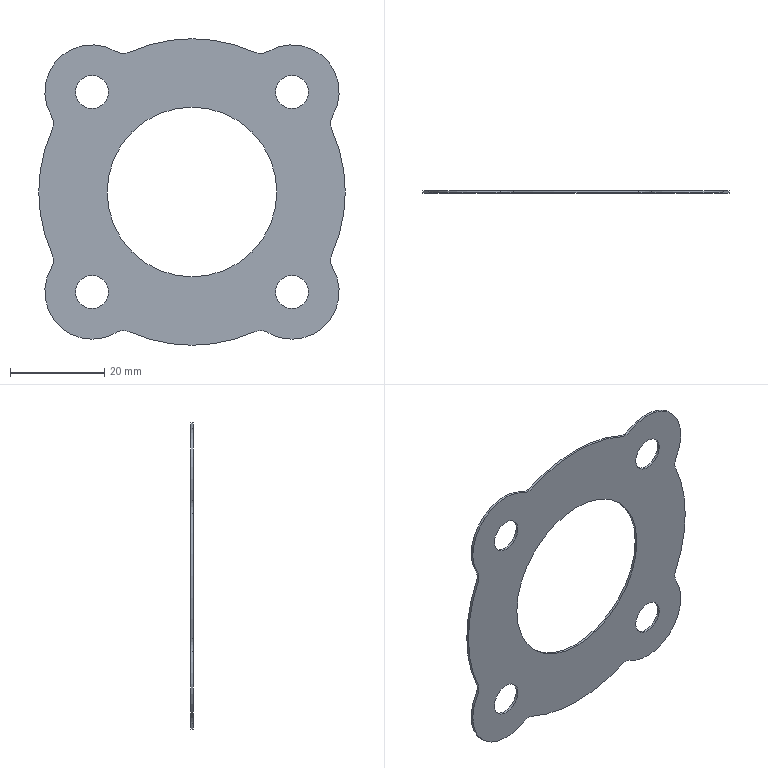Part | SolidWorks | features Extrusion 1, Fillet 1, ICE 1 | 1 solid | 33 faces | box 65 x 0.5 x 65 mm | volume 1310 mm3 | cylinder 31 | plane 2 | commonest cylinder face diameters 6 x10 7 x8 20 x6 65 x5 36 x2
STEP:
#1=CARTESIAN_POINT('',(14.555,0.,-29.379));
#2=VERTEX_POINT('',#1);
#3=CARTESIAN_POINT('',(16.092,0.,-29.802));
#4=VERTEX_POINT('',#3);
#5=CARTESIAN_POINT('',(14.555,0.,-32.379));
#6=DIRECTION('',(0.,1.,0.));
#7=DIRECTION('',(0.,0.,1.));
#8=AXIS2_PLACEMENT_3D('',#5,#6,#7);
#9=CIRCLE('',#8,3.);
#10=EDGE_CURVE('',#2,#4,#9,.T.);
#11=ORIENTED_EDGE('',*,*,#10,.F.);
#12=CARTESIAN_POINT('',(14.555,0.5,-29.379));
#13=VERTEX_POINT('',#12);
#14=CARTESIAN_POINT('',(14.555,0.5,-29.379));
#15=DIRECTION('',(0.,1.,0.));
#16=VECTOR('',#15,1000.);
#17=LINE('',#14,#16);
#18=EDGE_CURVE('',#2,#13,#17,.T.);
#19=ORIENTED_EDGE('',*,*,#18,.T.);
#20=CARTESIAN_POINT('',(16.092,0.5,-29.802));
#21=VERTEX_POINT('',#20);
#22=CARTESIAN_POINT('',(14.555,0.5,-32.379));
#23=DIRECTION('',(0.,-1.,0.));
#24=DIRECTION('',(0.,0.,1.));
#25=AXIS2_PLACEMENT_3D('',#22,#23,#24);
#26=CIRCLE('',#25,3.);
#27=EDGE_CURVE('',#21,#13,#26,.T.);
#28=ORIENTED_EDGE('',*,*,#27,.F.);
#29=CARTESIAN_POINT('',(16.092,0.5,-29.802));
#30=DIRECTION('',(0.,1.,0.));
#31=VECTOR('',#30,1000.);
#32=LINE('',#29,#31);
#33=EDGE_CURVE('',#4,#21,#32,.T.);
#34=ORIENTED_EDGE('',*,*,#33,.F.);
#35=EDGE_LOOP('',(#11,#19,#28,#34));
#36=FACE_OUTER_BOUND('',#35,.T.);
#37=CARTESIAN_POINT('',(14.555,0.5,-32.379));
#38=DIRECTION('',(0.,1.,0.));
#39=DIRECTION('',(0.,0.,1.));
#40=AXIS2_PLACEMENT_3D('',#37,#38,#39);
#41=CYLINDRICAL_SURFACE('',#40,3.);
#42=ADVANCED_FACE('',(#36),#41,.F.);
#43=CARTESIAN_POINT('',(-14.555,0.,-29.379));
#44=VERTEX_POINT('',#43);
#45=CARTESIAN_POINT('',(-13.325,0.,-29.643));
#46=VERTEX_POINT('',#45);
#47=CARTESIAN_POINT('',(-14.555,0.,-32.379));
#48=DIRECTION('',(0.,1.,0.));
#49=DIRECTION('',(0.,0.,1.));
#50=AXIS2_PLACEMENT_3D('',#47,#48,#49);
#51=CIRCLE('',#50,3.);
#52=EDGE_CURVE('',#44,#46,#51,.T.);
#53=ORIENTED_EDGE('',*,*,#52,.F.);
#54=CARTESIAN_POINT('',(-14.555,0.5,-29.379));
#55=VERTEX_POINT('',#54);
#56=CARTESIAN_POINT('',(-14.555,0.5,-29.379));
#57=DIRECTION('',(0.,1.,0.));
#58=VECTOR('',#57,1000.);
#59=LINE('',#56,#58);
#60=EDGE_CURVE('',#44,#55,#59,.T.);
#61=ORIENTED_EDGE('',*,*,#60,.T.);
#62=CARTESIAN_POINT('',(-13.325,0.5,-29.643));
#63=VERTEX_POINT('',#62);
#64=CARTESIAN_POINT('',(-14.555,0.5,-32.379));
#65=DIRECTION('',(0.,-1.,0.));
#66=DIRECTION('',(0.,0.,1.));
#67=AXIS2_PLACEMENT_3D('',#64,#65,#66);
#68=CIRCLE('',#67,3.);
#69=EDGE_CURVE('',#63,#55,#68,.T.);
#70=ORIENTED_EDGE('',*,*,#69,.F.);
#71=CARTESIAN_POINT('',(-13.325,0.5,-29.643));
#72=DIRECTION('',(0.,1.,0.));
#73=VECTOR('',#72,1000.);
#74=LINE('',#71,#73);
#75=EDGE_CURVE('',#46,#63,#74,.T.);
#76=ORIENTED_EDGE('',*,*,#75,.F.);
#77=EDGE_LOOP('',(#53,#61,#70,#76));
#78=FACE_OUTER_BOUND('',#77,.T.);
#79=CARTESIAN_POINT('',(-14.555,0.5,-32.379));
#80=DIRECTION('',(0.,1.,0.));
#81=DIRECTION('',(0.,0.,1.));
#82=AXIS2_PLACEMENT_3D('',#79,#80,#81);
#83=CYLINDRICAL_SURFACE('',#82,3.);
#84=ADVANCED_FACE('',(#78),#83,.F.);
#85=CARTESIAN_POINT('',(-21.213,0.,-24.713));
#86=VERTEX_POINT('',#85);
#87=CARTESIAN_POINT('',(-21.213,0.,-17.713));
#88=VERTEX_POINT('',#87);
#89=CARTESIAN_POINT('',(-21.213,0.,-21.213));
#90=DIRECTION('',(0.,1.,0.));
#91=DIRECTION('',(0.,0.,1.));
#92=AXIS2_PLACEMENT_3D('',#89,#90,#91);
#93=CIRCLE('',#92,3.5);
#94=EDGE_CURVE('',#86,#88,#93,.T.);
#95=ORIENTED_EDGE('',*,*,#94,.F.);
#96=CARTESIAN_POINT('',(-21.213,0.5,-24.713));
#97=VERTEX_POINT('',#96);
#98=CARTESIAN_POINT('',(-21.213,-49.5,-24.713));
#99=DIRECTION('',(0.,1.,0.));
#100=VECTOR('',#99,1000.);
#101=LINE('',#98,#100);
#102=EDGE_CURVE('',#86,#97,#101,.T.);
#103=ORIENTED_EDGE('',*,*,#102,.T.);
#104=CARTESIAN_POINT('',(-21.213,0.5,-17.713));
#105=VERTEX_POINT('',#104);
#106=CARTESIAN_POINT('',(-21.213,0.5,-21.213));
#107=DIRECTION('',(0.,1.,0.));
#108=DIRECTION('',(0.,0.,1.));
#109=AXIS2_PLACEMENT_3D('',#106,#107,#108);
#110=CIRCLE('',#109,3.5);
#111=EDGE_CURVE('',#97,#105,#110,.T.);
#112=ORIENTED_EDGE('',*,*,#111,.T.);
#113=CARTESIAN_POINT('',(-21.213,-49.5,-17.713));
#114=DIRECTION('',(0.,1.,0.));
#115=VECTOR('',#114,1000.);
#116=LINE('',#113,#115);
#117=EDGE_CURVE('',#88,#105,#116,.T.);
#118=ORIENTED_EDGE('',*,*,#117,.F.);
#119=EDGE_LOOP('',(#95,#103,#112,#118));
#120=FACE_OUTER_BOUND('',#119,.T.);
#121=CARTESIAN_POINT('',(-21.213,-49.5,-21.213));
#122=DIRECTION('',(0.,1.,0.));
#123=DIRECTION('',(0.,0.,1.));
#124=AXIS2_PLACEMENT_3D('',#121,#122,#123);
#125=CYLINDRICAL_SURFACE('',#124,3.5);
#126=ADVANCED_FACE('',(#120),#125,.F.);
#127=CARTESIAN_POINT('',(-21.213,0.,17.713));
#128=VERTEX_POINT('',#127);
#129=CARTESIAN_POINT('',(-21.213,0.,24.713));
#130=VERTEX_POINT('',#129);
#131=CARTESIAN_POINT('',(-21.213,0.,21.213));
#132=DIRECTION('',(0.,1.,0.));
#133=DIRECTION('',(0.,0.,1.));
#134=AXIS2_PLACEMENT_3D('',#131,#132,#133);
#135=CIRCLE('',#134,3.5);
#136=EDGE_CURVE('',#128,#130,#135,.T.);
#137=ORIENTED_EDGE('',*,*,#136,.F.);
#138=CARTESIAN_POINT('',(-21.213,0.5,17.713));
#139=VERTEX_POINT('',#138);
#140=CARTESIAN_POINT('',(-21.213,-49.5,17.713));
#141=DIRECTION('',(0.,1.,0.));
#142=VECTOR('',#141,1000.);
#143=LINE('',#140,#142);
#144=EDGE_CURVE('',#128,#139,#143,.T.);
#145=ORIENTED_EDGE('',*,*,#144,.T.);
#146=CARTESIAN_POINT('',(-21.213,0.5,24.713));
#147=VERTEX_POINT('',#146);
#148=CARTESIAN_POINT('',(-21.213,0.5,21.213));
#149=DIRECTION('',(0.,1.,0.));
#150=DIRECTION('',(0.,0.,1.));
#151=AXIS2_PLACEMENT_3D('',#148,#149,#150);
#152=CIRCLE('',#151,3.5);
#153=EDGE_CURVE('',#139,#147,#152,.T.);
#154=ORIENTED_EDGE('',*,*,#153,.T.);
#155=CARTESIAN_POINT('',(-21.213,-49.5,24.713));
#156=DIRECTION('',(0.,1.,0.));
#157=VECTOR('',#156,1000.);
#158=LINE('',#155,#157);
#159=EDGE_CURVE('',#130,#147,#158,.T.);
#160=ORIENTED_EDGE('',*,*,#159,.F.);
#161=EDGE_LOOP('',(#137,#145,#154,#160));
#162=FACE_OUTER_BOUND('',#161,.T.);
#163=CARTESIAN_POINT('',(-21.213,-49.5,21.213));
#164=DIRECTION('',(0.,1.,0.));
#165=DIRECTION('',(0.,0.,1.));
#166=AXIS2_PLACEMENT_3D('',#163,#164,#165);
#167=CYLINDRICAL_SURFACE('',#166,3.5);
#168=ADVANCED_FACE('',(#162),#167,.F.);
#169=CARTESIAN_POINT('',(21.213,0.,17.713));
#170=VERTEX_POINT('',#169);
#171=CARTESIAN_POINT('',(21.213,0.,24.713));
#172=VERTEX_POINT('',#171);
#173=CARTESIAN_POINT('',(21.213,0.,21.213));
#174=DIRECTION('',(0.,1.,0.));
#175=DIRECTION('',(0.,0.,1.));
#176=AXIS2_PLACEMENT_3D('',#173,#174,#175);
#177=CIRCLE('',#176,3.5);
#178=EDGE_CURVE('',#170,#172,#177,.T.);
#179=ORIENTED_EDGE('',*,*,#178,.F.);
#180=CARTESIAN_POINT('',(21.213,0.5,17.713));
#181=VERTEX_POINT('',#180);
#182=CARTESIAN_POINT('',(21.213,-49.5,17.713));
#183=DIRECTION('',(0.,1.,0.));
#184=VECTOR('',#183,1000.);
#185=LINE('',#182,#184);
#186=EDGE_CURVE('',#170,#181,#185,.T.);
#187=ORIENTED_EDGE('',*,*,#186,.T.);
#188=CARTESIAN_POINT('',(21.213,0.5,24.713));
#189=VERTEX_POINT('',#188);
#190=CARTESIAN_POINT('',(21.213,0.5,21.213));
#191=DIRECTION('',(0.,1.,0.));
#192=DIRECTION('',(0.,0.,1.));
#193=AXIS2_PLACEMENT_3D('',#190,#191,#192);
#194=CIRCLE('',#193,3.5);
#195=EDGE_CURVE('',#181,#189,#194,.T.);
#196=ORIENTED_EDGE('',*,*,#195,.T.);
#197=CARTESIAN_POINT('',(21.213,-49.5,24.713));
#198=DIRECTION('',(0.,1.,0.));
#199=VECTOR('',#198,1000.);
#200=LINE('',#197,#199);
#201=EDGE_CURVE('',#172,#189,#200,.T.);
#202=ORIENTED_EDGE('',*,*,#201,.F.);
#203=EDGE_LOOP('',(#179,#187,#196,#202));
#204=FACE_OUTER_BOUND('',#203,.T.);
#205=CARTESIAN_POINT('',(21.213,-49.5,21.213));
#206=DIRECTION('',(0.,1.,0.));
#207=DIRECTION('',(0.,0.,1.));
#208=AXIS2_PLACEMENT_3D('',#205,#206,#207);
#209=CYLINDRICAL_SURFACE('',#208,3.5);
#210=ADVANCED_FACE('',(#204),#209,.F.);
#211=CARTESIAN_POINT('',(21.213,0.,-24.713));
#212=VERTEX_POINT('',#211);
#213=CARTESIAN_POINT('',(21.213,0.,-17.713));
#214=VERTEX_POINT('',#213);
#215=CARTESIAN_POINT('',(21.213,0.,-21.213));
#216=DIRECTION('',(0.,1.,0.));
#217=DIRECTION('',(0.,0.,1.));
#218=AXIS2_PLACEMENT_3D('',#215,#216,#217);
#219=CIRCLE('',#218,3.5);
#220=EDGE_CURVE('',#212,#214,#219,.T.);
#221=ORIENTED_EDGE('',*,*,#220,.F.);
#222=CARTESIAN_POINT('',(21.213,0.5,-24.713));
#223=VERTEX_POINT('',#222);
#224=CARTESIAN_POINT('',(21.213,-49.5,-24.713));
#225=DIRECTION('',(0.,1.,0.));
#226=VECTOR('',#225,1000.);
#227=LINE('',#224,#226);
#228=EDGE_CURVE('',#212,#223,#227,.T.);
#229=ORIENTED_EDGE('',*,*,#228,.T.);
#230=CARTESIAN_POINT('',(21.213,0.5,-17.713));
#231=VERTEX_POINT('',#230);
#232=CARTESIAN_POINT('',(21.213,0.5,-21.213));
#233=DIRECTION('',(0.,1.,0.));
#234=DIRECTION('',(0.,0.,1.));
#235=AXIS2_PLACEMENT_3D('',#232,#233,#234);
#236=CIRCLE('',#235,3.5);
#237=EDGE_CURVE('',#223,#231,#236,.T.);
#238=ORIENTED_EDGE('',*,*,#237,.T.);
#239=CARTESIAN_POINT('',(21.213,-49.5,-17.713));
#240=DIRECTION('',(0.,1.,0.));
#241=VECTOR('',#240,1000.);
#242=LINE('',#239,#241);
#243=EDGE_CURVE('',#214,#231,#242,.T.);
#244=ORIENTED_EDGE('',*,*,#243,.F.);
#245=EDGE_LOOP('',(#221,#229,#238,#244));
#246=FACE_OUTER_BOUND('',#245,.T.);
#247=CARTESIAN_POINT('',(21.213,-49.5,-21.213));
#248=DIRECTION('',(0.,1.,0.));
#249=DIRECTION('',(0.,0.,1.));
#250=AXIS2_PLACEMENT_3D('',#247,#248,#249);
#251=CYLINDRICAL_SURFACE('',#250,3.5);
#252=ADVANCED_FACE('',(#246),#251,.F.);
#253=CARTESIAN_POINT('',(0.,0.,-18.));
#254=VERTEX_POINT('',#253);
#255=CARTESIAN_POINT('',(0.,0.,18.));
#256=VERTEX_POINT('',#255);
#257=CARTESIAN_POINT('',(0.,0.,0.));
#258=DIRECTION('',(0.,1.,0.));
#259=DIRECTION('',(0.,0.,1.));
#260=AXIS2_PLACEMENT_3D('',#257,#258,#259);
#261=CIRCLE('',#260,18.);
#262=EDGE_CURVE('',#254,#256,#261,.T.);
#263=ORIENTED_EDGE('',*,*,#262,.F.);
#264=CARTESIAN_POINT('',(0.,0.5,-18.));
#265=VERTEX_POINT('',#264);
#266=CARTESIAN_POINT('',(0.,-49.5,-18.));
#267=DIRECTION('',(0.,1.,0.));
#268=VECTOR('',#267,1000.);
#269=LINE('',#266,#268);
#270=EDGE_CURVE('',#254,#265,#269,.T.);
#271=ORIENTED_EDGE('',*,*,#270,.T.);
#272=CARTESIAN_POINT('',(0.,0.5,18.));
#273=VERTEX_POINT('',#272);
#274=CARTESIAN_POINT('',(0.,0.5,0.));
#275=DIRECTION('',(0.,1.,0.));
#276=DIRECTION('',(0.,0.,1.));
#277=AXIS2_PLACEMENT_3D('',#274,#275,#276);
#278=CIRCLE('',#277,18.);
#279=EDGE_CURVE('',#265,#273,#278,.T.);
#280=ORIENTED_EDGE('',*,*,#279,.T.);
#281=CARTESIAN_POINT('',(0.,-49.5,18.));
#282=DIRECTION('',(0.,1.,0.));
#283=VECTOR('',#282,1000.);
#284=LINE('',#281,#283);
#285=EDGE_CURVE('',#256,#273,#284,.T.);
#286=ORIENTED_EDGE('',*,*,#285,.F.);
#287=EDGE_LOOP('',(#263,#271,#280,#286));
#288=FACE_OUTER_BOUND('',#287,.T.);
#289=CARTESIAN_POINT('',(0.,-49.5,0.));
#290=DIRECTION('',(0.,1.,0.));
#291=DIRECTION('',(0.,0.,1.));
#292=AXIS2_PLACEMENT_3D('',#289,#290,#291);
#293=CYLINDRICAL_SURFACE('',#292,18.);
#294=ADVANCED_FACE('',(#288),#293,.F.);
#295=CARTESIAN_POINT('',(-21.213,0.5,-31.213));
#296=VERTEX_POINT('',#295);
#297=CARTESIAN_POINT('',(-29.802,0.5,-16.092));
#298=VERTEX_POINT('',#297);
#299=CARTESIAN_POINT('',(-21.213,0.5,-21.213));
#300=DIRECTION('',(0.,1.,0.));
#301=DIRECTION('',(0.,0.,1.));
#302=AXIS2_PLACEMENT_3D('',#299,#300,#301);
#303=CIRCLE('',#302,10.);
#304=EDGE_CURVE('',#296,#298,#303,.T.);
#305=ORIENTED_EDGE('',*,*,#304,.F.);
#306=CARTESIAN_POINT('',(-21.213,0.,-31.213));
#307=VERTEX_POINT('',#306);
#308=CARTESIAN_POINT('',(-21.213,0.5,-31.213));
#309=DIRECTION('',(0.,-1.,0.));
#310=VECTOR('',#309,1000.);
#311=LINE('',#308,#310);
#312=EDGE_CURVE('',#296,#307,#311,.T.);
#313=ORIENTED_EDGE('',*,*,#312,.T.);
#314=CARTESIAN_POINT('',(-29.802,0.,-16.092));
#315=VERTEX_POINT('',#314);
#316=CARTESIAN_POINT('',(-21.213,0.,-21.213));
#317=DIRECTION('',(0.,1.,0.));
#318=DIRECTION('',(0.,0.,1.));
#319=AXIS2_PLACEMENT_3D('',#316,#317,#318);
#320=CIRCLE('',#319,10.);
#321=EDGE_CURVE('',#307,#315,#320,.T.);
#322=ORIENTED_EDGE('',*,*,#321,.T.);
#323=CARTESIAN_POINT('',(-29.802,0.5,-16.092));
#324=DIRECTION('',(0.,1.,0.));
#325=VECTOR('',#324,1000.);
#326=LINE('',#323,#325);
#327=EDGE_CURVE('',#315,#298,#326,.T.);
#328=ORIENTED_EDGE('',*,*,#327,.T.);
#329=EDGE_LOOP('',(#305,#313,#322,#328));
#330=FACE_OUTER_BOUND('',#329,.T.);
#331=CARTESIAN_POINT('',(-21.213,0.5,-21.213));
#332=DIRECTION('',(0.,-1.,0.));
#333=DIRECTION('',(0.,0.,-1.));
#334=AXIS2_PLACEMENT_3D('',#331,#332,#333);
#335=CYLINDRICAL_SURFACE('',#334,10.);
#336=ADVANCED_FACE('',(#330),#335,.T.);
#337=CARTESIAN_POINT('',(0.,0.5,-32.5));
#338=VERTEX_POINT('',#337);
#339=CARTESIAN_POINT('',(0.,0.5,0.));
#340=DIRECTION('',(0.,1.,0.));
#341=DIRECTION('',(0.,0.,1.));
#342=AXIS2_PLACEMENT_3D('',#339,#340,#341);
#343=CIRCLE('',#342,32.5);
#344=EDGE_CURVE('',#338,#63,#343,.T.);
#345=ORIENTED_EDGE('',*,*,#344,.F.);
#346=CARTESIAN_POINT('',(0.,0.,-32.5));
#347=VERTEX_POINT('',#346);
#348=CARTESIAN_POINT('',(0.,0.5,-32.5));
#349=DIRECTION('',(0.,-1.,0.));
#350=VECTOR('',#349,1000.);
#351=LINE('',#348,#350);
#352=EDGE_CURVE('',#338,#347,#351,.T.);
#353=ORIENTED_EDGE('',*,*,#352,.T.);
#354=CARTESIAN_POINT('',(0.,0.,0.));
#355=DIRECTION('',(0.,1.,0.));
#356=DIRECTION('',(0.,0.,1.));
#357=AXIS2_PLACEMENT_3D('',#354,#355,#356);
#358=CIRCLE('',#357,32.5);
#359=EDGE_CURVE('',#347,#46,#358,.T.);
#360=ORIENTED_EDGE('',*,*,#359,.T.);
#361=ORIENTED_EDGE('',*,*,#75,.T.);
#362=EDGE_LOOP('',(#345,#353,#360,#361));
#363=FACE_OUTER_BOUND('',#362,.T.);
#364=CARTESIAN_POINT('',(0.,0.5,0.));
#365=DIRECTION('',(0.,-1.,0.));
#366=DIRECTION('',(0.,0.,-1.));
#367=AXIS2_PLACEMENT_3D('',#364,#365,#366);
#368=CYLINDRICAL_SURFACE('',#367,32.5);
#369=ADVANCED_FACE('',(#363),#368,.T.);
#370=CARTESIAN_POINT('',(21.213,0.5,-31.213));
#371=VERTEX_POINT('',#370);
#372=CARTESIAN_POINT('',(21.213,0.5,-21.213));
#373=DIRECTION('',(0.,1.,0.));
#374=DIRECTION('',(0.,0.,1.));
#375=AXIS2_PLACEMENT_3D('',#372,#373,#374);
#376=CIRCLE('',#375,10.);
#377=EDGE_CURVE('',#371,#21,#376,.T.);
#378=ORIENTED_EDGE('',*,*,#377,.F.);
#379=CARTESIAN_POINT('',(21.213,0.,-31.213));
#380=VERTEX_POINT('',#379);
#381=CARTESIAN_POINT('',(21.213,0.5,-31.213));
#382=DIRECTION('',(0.,-1.,0.));
#383=VECTOR('',#382,1000.);
#384=LINE('',#381,#383);
#385=EDGE_CURVE('',#371,#380,#384,.T.);
#386=ORIENTED_EDGE('',*,*,#385,.T.);
#387=CARTESIAN_POINT('',(21.213,0.,-21.213));
#388=DIRECTION('',(0.,1.,0.));
#389=DIRECTION('',(0.,0.,1.));
#390=AXIS2_PLACEMENT_3D('',#387,#388,#389);
#391=CIRCLE('',#390,10.);
#392=EDGE_CURVE('',#380,#4,#391,.T.);
#393=ORIENTED_EDGE('',*,*,#392,.T.);
#394=ORIENTED_EDGE('',*,*,#33,.T.);
#395=EDGE_LOOP('',(#378,#386,#393,#394));
#396=FACE_OUTER_BOUND('',#395,.T.);
#397=CARTESIAN_POINT('',(21.213,0.5,-21.213));
#398=DIRECTION('',(0.,-1.,0.));
#399=DIRECTION('',(0.,0.,-1.));
#400=AXIS2_PLACEMENT_3D('',#397,#398,#399);
#401=CYLINDRICAL_SURFACE('',#400,10.);
#402=ADVANCED_FACE('',(#396),#401,.T.);
#403=CARTESIAN_POINT('',(-29.643,0.5,-13.325));
#404=VERTEX_POINT('',#403);
#405=CARTESIAN_POINT('',(-29.643,0.5,13.325));
#406=VERTEX_POINT('',#405);
#407=CARTESIAN_POINT('',(0.,0.5,0.));
#408=DIRECTION('',(0.,1.,0.));
#409=DIRECTION('',(0.,0.,1.));
#410=AXIS2_PLACEMENT_3D('',#407,#408,#409);
#411=CIRCLE('',#410,32.5);
#412=EDGE_CURVE('',#404,#406,#411,.T.);
#413=ORIENTED_EDGE('',*,*,#412,.F.);
#414=CARTESIAN_POINT('',(-29.643,0.,-13.325));
#415=VERTEX_POINT('',#414);
#416=CARTESIAN_POINT('',(-29.643,0.5,-13.325));
#417=DIRECTION('',(0.,-1.,0.));
#418=VECTOR('',#417,1000.);
#419=LINE('',#416,#418);
#420=EDGE_CURVE('',#404,#415,#419,.T.);
#421=ORIENTED_EDGE('',*,*,#420,.T.);
#422=CARTESIAN_POINT('',(-29.643,0.,13.325));
#423=VERTEX_POINT('',#422);
#424=CARTESIAN_POINT('',(0.,0.,0.));
#425=DIRECTION('',(0.,1.,0.));
#426=DIRECTION('',(0.,0.,1.));
#427=AXIS2_PLACEMENT_3D('',#424,#425,#426);
#428=CIRCLE('',#427,32.5);
#429=EDGE_CURVE('',#415,#423,#428,.T.);
#430=ORIENTED_EDGE('',*,*,#429,.T.);
#431=CARTESIAN_POINT('',(-29.643,0.5,13.325));
#432=DIRECTION('',(0.,1.,0.));
#433=VECTOR('',#432,1000.);
#434=LINE('',#431,#433);
#435=EDGE_CURVE('',#423,#406,#434,.T.);
#436=ORIENTED_EDGE('',*,*,#435,.T.);
#437=EDGE_LOOP('',(#413,#421,#430,#436));
#438=FACE_OUTER_BOUND('',#437,.T.);
#439=CARTESIAN_POINT('',(0.,0.5,0.));
#440=DIRECTION('',(0.,-1.,0.));
#441=DIRECTION('',(0.,0.,-1.));
#442=AXIS2_PLACEMENT_3D('',#439,#440,#441);
#443=CYLINDRICAL_SURFACE('',#442,32.5);
#444=ADVANCED_FACE('',(#438),#443,.T.);
#445=CARTESIAN_POINT('',(-29.802,0.,16.092));
#446=VERTEX_POINT('',#445);
#447=CARTESIAN_POINT('',(-16.092,0.,29.802));
#448=VERTEX_POINT('',#447);
#449=CARTESIAN_POINT('',(-21.213,0.,21.213));
#450=DIRECTION('',(0.,1.,0.));
#451=DIRECTION('',(0.,0.,1.));
#452=AXIS2_PLACEMENT_3D('',#449,#450,#451);
#453=CIRCLE('',#452,10.);
#454=EDGE_CURVE('',#446,#448,#453,.T.);
#455=ORIENTED_EDGE('',*,*,#454,.T.);
#456=CARTESIAN_POINT('',(-16.092,0.5,29.802));
#457=VERTEX_POINT('',#456);
#458=CARTESIAN_POINT('',(-16.092,0.5,29.802));
#459=DIRECTION('',(0.,1.,0.));
#460=VECTOR('',#459,1000.);
#461=LINE('',#458,#460);
#462=EDGE_CURVE('',#448,#457,#461,.T.);
#463=ORIENTED_EDGE('',*,*,#462,.T.);
#464=CARTESIAN_POINT('',(-29.802,0.5,16.092));
#465=VERTEX_POINT('',#464);
#466=CARTESIAN_POINT('',(-21.213,0.5,21.213));
#467=DIRECTION('',(0.,1.,0.));
#468=DIRECTION('',(0.,0.,1.));
#469=AXIS2_PLACEMENT_3D('',#466,#467,#468);
#470=CIRCLE('',#469,10.);
#471=EDGE_CURVE('',#465,#457,#470,.T.);
#472=ORIENTED_EDGE('',*,*,#471,.F.);
#473=CARTESIAN_POINT('',(-29.802,0.5,16.092));
#474=DIRECTION('',(0.,-1.,0.));
#475=VECTOR('',#474,1000.);
#476=LINE('',#473,#475);
#477=EDGE_CURVE('',#465,#446,#476,.T.);
#478=ORIENTED_EDGE('',*,*,#477,.T.);
#479=EDGE_LOOP('',(#455,#463,#472,#478));
#480=FACE_OUTER_BOUND('',#479,.T.);
#481=CARTESIAN_POINT('',(-21.213,0.5,21.213));
#482=DIRECTION('',(0.,-1.,0.));
#483=DIRECTION('',(0.,0.,-1.));
#484=AXIS2_PLACEMENT_3D('',#481,#482,#483);
#485=CYLINDRICAL_SURFACE('',#484,10.);
#486=ADVANCED_FACE('',(#480),#485,.T.);
#487=CARTESIAN_POINT('',(-13.325,0.5,29.643));
#488=VERTEX_POINT('',#487);
#489=CARTESIAN_POINT('',(13.325,0.5,29.643));
#490=VERTEX_POINT('',#489);
#491=CARTESIAN_POINT('',(0.,0.5,0.));
#492=DIRECTION('',(0.,1.,0.));
#493=DIRECTION('',(0.,0.,1.));
#494=AXIS2_PLACEMENT_3D('',#491,#492,#493);
#495=CIRCLE('',#494,32.5);
#496=EDGE_CURVE('',#488,#490,#495,.T.);
#497=ORIENTED_EDGE('',*,*,#496,.F.);
#498=CARTESIAN_POINT('',(-13.325,0.,29.643));
#499=VERTEX_POINT('',#498);
#500=CARTESIAN_POINT('',(-13.325,0.5,29.643));
#501=DIRECTION('',(0.,-1.,0.));
#502=VECTOR('',#501,1000.);
#503=LINE('',#500,#502);
#504=EDGE_CURVE('',#488,#499,#503,.T.);
#505=ORIENTED_EDGE('',*,*,#504,.T.);
#506=CARTESIAN_POINT('',(13.325,0.,29.643));
#507=VERTEX_POINT('',#506);
#508=CARTESIAN_POINT('',(0.,0.,0.));
#509=DIRECTION('',(0.,1.,0.));
#510=DIRECTION('',(0.,0.,1.));
#511=AXIS2_PLACEMENT_3D('',#508,#509,#510);
#512=CIRCLE('',#511,32.5);
#513=EDGE_CURVE('',#499,#507,#512,.T.);
#514=ORIENTED_EDGE('',*,*,#513,.T.);
#515=CARTESIAN_POINT('',(13.325,0.5,29.643));
#516=DIRECTION('',(0.,1.,0.));
#517=VECTOR('',#516,1000.);
#518=LINE('',#515,#517);
#519=EDGE_CURVE('',#507,#490,#518,.T.);
#520=ORIENTED_EDGE('',*,*,#519,.T.);
#521=EDGE_LOOP('',(#497,#505,#514,#520));
#522=FACE_OUTER_BOUND('',#521,.T.);
#523=CARTESIAN_POINT('',(0.,0.5,0.));
#524=DIRECTION('',(0.,-1.,0.));
#525=DIRECTION('',(0.,0.,-1.));
#526=AXIS2_PLACEMENT_3D('',#523,#524,#525);
#527=CYLINDRICAL_SURFACE('',#526,32.5);
#528=ADVANCED_FACE('',(#522),#527,.T.);
#529=CARTESIAN_POINT('',(16.092,0.,29.802));
#530=VERTEX_POINT('',#529);
#531=CARTESIAN_POINT('',(29.802,0.,16.092));
#532=VERTEX_POINT('',#531);
#533=CARTESIAN_POINT('',(21.213,0.,21.213));
#534=DIRECTION('',(0.,1.,0.));
#535=DIRECTION('',(0.,0.,1.));
#536=AXIS2_PLACEMENT_3D('',#533,#534,#535);
#537=CIRCLE('',#536,10.);
#538=EDGE_CURVE('',#530,#532,#537,.T.);
#539=ORIENTED_EDGE('',*,*,#538,.T.);
#540=CARTESIAN_POINT('',(29.802,0.5,16.092));
#541=VERTEX_POINT('',#540);
#542=CARTESIAN_POINT('',(29.802,0.5,16.092));
#543=DIRECTION('',(0.,1.,0.));
#544=VECTOR('',#543,1000.);
#545=LINE('',#542,#544);
#546=EDGE_CURVE('',#532,#541,#545,.T.);
#547=ORIENTED_EDGE('',*,*,#546,.T.);
#548=CARTESIAN_POINT('',(16.092,0.5,29.802));
#549=VERTEX_POINT('',#548);
#550=CARTESIAN_POINT('',(21.213,0.5,21.213));
#551=DIRECTION('',(0.,1.,0.));
#552=DIRECTION('',(0.,0.,1.));
#553=AXIS2_PLACEMENT_3D('',#550,#551,#552);
#554=CIRCLE('',#553,10.);
#555=EDGE_CURVE('',#549,#541,#554,.T.);
#556=ORIENTED_EDGE('',*,*,#555,.F.);
#557=CARTESIAN_POINT('',(16.092,0.5,29.802));
#558=DIRECTION('',(0.,-1.,0.));
#559=VECTOR('',#558,1000.);
#560=LINE('',#557,#559);
#561=EDGE_CURVE('',#549,#530,#560,.T.);
#562=ORIENTED_EDGE('',*,*,#561,.T.);
#563=EDGE_LOOP('',(#539,#547,#556,#562));
#564=FACE_OUTER_BOUND('',#563,.T.);
#565=CARTESIAN_POINT('',(21.213,0.5,21.213));
#566=DIRECTION('',(0.,-1.,0.));
#567=DIRECTION('',(0.,0.,-1.));
#568=AXIS2_PLACEMENT_3D('',#565,#566,#567);
#569=CYLINDRICAL_SURFACE('',#568,10.);
#570=ADVANCED_FACE('',(#564),#569,.T.);
#571=CARTESIAN_POINT('',(29.643,0.,13.325));
#572=VERTEX_POINT('',#571);
#573=CARTESIAN_POINT('',(29.643,0.,-13.325));
#574=VERTEX_POINT('',#573);
#575=CARTESIAN_POINT('',(0.,0.,0.));
#576=DIRECTION('',(0.,1.,0.));
#577=DIRECTION('',(0.,0.,1.));
#578=AXIS2_PLACEMENT_3D('',#575,#576,#577);
#579=CIRCLE('',#578,32.5);
#580=EDGE_CURVE('',#572,#574,#579,.T.);
#581=ORIENTED_EDGE('',*,*,#580,.T.);
#582=CARTESIAN_POINT('',(29.643,0.5,-13.325));
#583=VERTEX_POINT('',#582);
#584=CARTESIAN_POINT('',(29.643,0.5,-13.325));
#585=DIRECTION('',(0.,1.,0.));
#586=VECTOR('',#585,1000.);
#587=LINE('',#584,#586);
#588=EDGE_CURVE('',#574,#583,#587,.T.);
#589=ORIENTED_EDGE('',*,*,#588,.T.);
#590=CARTESIAN_POINT('',(29.643,0.5,13.325));
#591=VERTEX_POINT('',#590);
#592=CARTESIAN_POINT('',(0.,0.5,0.));
#593=DIRECTION('',(0.,1.,0.));
#594=DIRECTION('',(0.,0.,1.));
#595=AXIS2_PLACEMENT_3D('',#592,#593,#594);
#596=CIRCLE('',#595,32.5);
#597=EDGE_CURVE('',#591,#583,#596,.T.);
#598=ORIENTED_EDGE('',*,*,#597,.F.);
#599=CARTESIAN_POINT('',(29.643,0.5,13.325));
#600=DIRECTION('',(0.,-1.,0.));
#601=VECTOR('',#600,1000.);
#602=LINE('',#599,#601);
#603=EDGE_CURVE('',#591,#572,#602,.T.);
#604=ORIENTED_EDGE('',*,*,#603,.T.);
#605=EDGE_LOOP('',(#581,#589,#598,#604));
#606=FACE_OUTER_BOUND('',#605,.T.);
#607=CARTESIAN_POINT('',(0.,0.5,0.));
#608=DIRECTION('',(0.,-1.,0.));
#609=DIRECTION('',(0.,0.,-1.));
#610=AXIS2_PLACEMENT_3D('',#607,#608,#609);
#611=CYLINDRICAL_SURFACE('',#610,32.5);
#612=ADVANCED_FACE('',(#606),#611,.T.);
#613=ORIENTED_EDGE('',*,*,#385,.F.);
#614=CARTESIAN_POINT('',(29.802,0.5,-16.092));
#615=VERTEX_POINT('',#614);
#616=CARTESIAN_POINT('',(21.213,0.5,-21.213));
#617=DIRECTION('',(0.,1.,0.));
#618=DIRECTION('',(0.,0.,1.));
#619=AXIS2_PLACEMENT_3D('',#616,#617,#618);
#620=CIRCLE('',#619,10.);
#621=EDGE_CURVE('',#615,#371,#620,.T.);
#622=ORIENTED_EDGE('',*,*,#621,.F.);
#623=CARTESIAN_POINT('',(29.802,0.,-16.092));
#624=VERTEX_POINT('',#623);
#625=CARTESIAN_POINT('',(29.802,0.5,-16.092));
#626=DIRECTION('',(0.,-1.,0.));
#627=VECTOR('',#626,1000.);
#628=LINE('',#625,#627);
#629=EDGE_CURVE('',#615,#624,#628,.T.);
#630=ORIENTED_EDGE('',*,*,#629,.T.);
#631=CARTESIAN_POINT('',(21.213,0.,-21.213));
#632=DIRECTION('',(0.,1.,0.));
#633=DIRECTION('',(0.,0.,1.));
#634=AXIS2_PLACEMENT_3D('',#631,#632,#633);
#635=CIRCLE('',#634,10.);
#636=EDGE_CURVE('',#624,#380,#635,.T.);
#637=ORIENTED_EDGE('',*,*,#636,.T.);
#638=EDGE_LOOP('',(#613,#622,#630,#637));
#639=FACE_OUTER_BOUND('',#638,.T.);
#640=CARTESIAN_POINT('',(21.213,0.5,-21.213));
#641=DIRECTION('',(0.,-1.,0.));
#642=DIRECTION('',(0.,0.,-1.));
#643=AXIS2_PLACEMENT_3D('',#640,#641,#642);
#644=CYLINDRICAL_SURFACE('',#643,10.);
#645=ADVANCED_FACE('',(#639),#644,.T.);
#646=ORIENTED_EDGE('',*,*,#352,.F.);
#647=CARTESIAN_POINT('',(13.325,0.5,-29.643));
#648=VERTEX_POINT('',#647);
#649=CARTESIAN_POINT('',(0.,0.5,0.));
#650=DIRECTION('',(0.,1.,0.));
#651=DIRECTION('',(0.,0.,1.));
#652=AXIS2_PLACEMENT_3D('',#649,#650,#651);
#653=CIRCLE('',#652,32.5);
#654=EDGE_CURVE('',#648,#338,#653,.T.);
#655=ORIENTED_EDGE('',*,*,#654,.F.);
#656=CARTESIAN_POINT('',(13.325,0.,-29.643));
#657=VERTEX_POINT('',#656);
#658=CARTESIAN_POINT('',(13.325,0.5,-29.643));
#659=DIRECTION('',(0.,-1.,0.));
#660=VECTOR('',#659,1000.);
#661=LINE('',#658,#660);
#662=EDGE_CURVE('',#648,#657,#661,.T.);
#663=ORIENTED_EDGE('',*,*,#662,.T.);
#664=CARTESIAN_POINT('',(0.,0.,0.));
#665=DIRECTION('',(0.,1.,0.));
#666=DIRECTION('',(0.,0.,1.));
#667=AXIS2_PLACEMENT_3D('',#664,#665,#666);
#668=CIRCLE('',#667,32.5);
#669=EDGE_CURVE('',#657,#347,#668,.T.);
#670=ORIENTED_EDGE('',*,*,#669,.T.);
#671=EDGE_LOOP('',(#646,#655,#663,#670));
#672=FACE_OUTER_BOUND('',#671,.T.);
#673=CARTESIAN_POINT('',(0.,0.5,0.));
#674=DIRECTION('',(0.,-1.,0.));
#675=DIRECTION('',(0.,0.,-1.));
#676=AXIS2_PLACEMENT_3D('',#673,#674,#675);
#677=CYLINDRICAL_SURFACE('',#676,32.5);
#678=ADVANCED_FACE('',(#672),#677,.T.);
#679=ORIENTED_EDGE('',*,*,#312,.F.);
#680=CARTESIAN_POINT('',(-16.092,0.5,-29.802));
#681=VERTEX_POINT('',#680);
#682=CARTESIAN_POINT('',(-21.213,0.5,-21.213));
#683=DIRECTION('',(0.,1.,0.));
#684=DIRECTION('',(0.,0.,1.));
#685=AXIS2_PLACEMENT_3D('',#682,#683,#684);
#686=CIRCLE('',#685,10.);
#687=EDGE_CURVE('',#681,#296,#686,.T.);
#688=ORIENTED_EDGE('',*,*,#687,.F.);
#689=CARTESIAN_POINT('',(-16.092,0.,-29.802));
#690=VERTEX_POINT('',#689);
#691=CARTESIAN_POINT('',(-16.092,0.5,-29.802));
#692=DIRECTION('',(0.,-1.,0.));
#693=VECTOR('',#692,1000.);
#694=LINE('',#691,#693);
#695=EDGE_CURVE('',#681,#690,#694,.T.);
#696=ORIENTED_EDGE('',*,*,#695,.T.);
#697=CARTESIAN_POINT('',(-21.213,0.,-21.213));
#698=DIRECTION('',(0.,1.,0.));
#699=DIRECTION('',(0.,0.,1.));
#700=AXIS2_PLACEMENT_3D('',#697,#698,#699);
#701=CIRCLE('',#700,10.);
#702=EDGE_CURVE('',#690,#307,#701,.T.);
#703=ORIENTED_EDGE('',*,*,#702,.T.);
#704=EDGE_LOOP('',(#679,#688,#696,#703));
#705=FACE_OUTER_BOUND('',#704,.T.);
#706=CARTESIAN_POINT('',(-21.213,0.5,-21.213));
#707=DIRECTION('',(0.,-1.,0.));
#708=DIRECTION('',(0.,0.,-1.));
#709=AXIS2_PLACEMENT_3D('',#706,#707,#708);
#710=CYLINDRICAL_SURFACE('',#709,10.);
#711=ADVANCED_FACE('',(#705),#710,.T.);
#712=CARTESIAN_POINT('',(-21.213,0.5,-21.213));
#713=DIRECTION('',(0.,1.,0.));
#714=DIRECTION('',(0.,0.,1.));
#715=AXIS2_PLACEMENT_3D('',#712,#713,#714);
#716=CIRCLE('',#715,3.5);
#717=EDGE_CURVE('',#105,#97,#716,.T.);
#718=ORIENTED_EDGE('',*,*,#717,.F.);
#719=ORIENTED_EDGE('',*,*,#111,.F.);
#720=EDGE_LOOP('',(#718,#719));
#721=FACE_BOUND('',#720,.T.);
#722=CARTESIAN_POINT('',(-21.213,0.5,21.213));
#723=DIRECTION('',(0.,1.,0.));
#724=DIRECTION('',(0.,0.,1.));
#725=AXIS2_PLACEMENT_3D('',#722,#723,#724);
#726=CIRCLE('',#725,3.5);
#727=EDGE_CURVE('',#147,#139,#726,.T.);
#728=ORIENTED_EDGE('',*,*,#727,.F.);
#729=ORIENTED_EDGE('',*,*,#153,.F.);
#730=EDGE_LOOP('',(#728,#729));
#731=FACE_BOUND('',#730,.T.);
#732=CARTESIAN_POINT('',(21.213,0.5,21.213));
#733=DIRECTION('',(0.,1.,0.));
#734=DIRECTION('',(0.,0.,1.));
#735=AXIS2_PLACEMENT_3D('',#732,#733,#734);
#736=CIRCLE('',#735,3.5);
#737=EDGE_CURVE('',#189,#181,#736,.T.);
#738=ORIENTED_EDGE('',*,*,#737,.F.);
#739=ORIENTED_EDGE('',*,*,#195,.F.);
#740=EDGE_LOOP('',(#738,#739));
#741=FACE_BOUND('',#740,.T.);
#742=CARTESIAN_POINT('',(21.213,0.5,-21.213));
#743=DIRECTION('',(0.,1.,0.));
#744=DIRECTION('',(0.,0.,1.));
#745=AXIS2_PLACEMENT_3D('',#742,#743,#744);
#746=CIRCLE('',#745,3.5);
#747=EDGE_CURVE('',#231,#223,#746,.T.);
#748=ORIENTED_EDGE('',*,*,#747,.F.);
#749=ORIENTED_EDGE('',*,*,#237,.F.);
#750=EDGE_LOOP('',(#748,#749));
#751=FACE_BOUND('',#750,.T.);
#752=CARTESIAN_POINT('',(0.,0.5,0.));
#753=DIRECTION('',(0.,1.,0.));
#754=DIRECTION('',(0.,0.,1.));
#755=AXIS2_PLACEMENT_3D('',#752,#753,#754);
#756=CIRCLE('',#755,18.);
#757=EDGE_CURVE('',#273,#265,#756,.T.);
#758=ORIENTED_EDGE('',*,*,#757,.F.);
#759=ORIENTED_EDGE('',*,*,#279,.F.);
#760=EDGE_LOOP('',(#758,#759));
#761=FACE_BOUND('',#760,.T.);
#762=ORIENTED_EDGE('',*,*,#687,.T.);
#763=ORIENTED_EDGE('',*,*,#304,.T.);
#764=CARTESIAN_POINT('',(-32.379,0.5,-14.555));
#765=DIRECTION('',(0.,-1.,0.));
#766=DIRECTION('',(0.,0.,1.));
#767=AXIS2_PLACEMENT_3D('',#764,#765,#766);
#768=CIRCLE('',#767,3.);
#769=EDGE_CURVE('',#298,#404,#768,.T.);
#770=ORIENTED_EDGE('',*,*,#769,.T.);
#771=ORIENTED_EDGE('',*,*,#412,.T.);
#772=CARTESIAN_POINT('',(-32.379,0.5,14.555));
#773=DIRECTION('',(0.,-1.,0.));
#774=DIRECTION('',(0.,0.,1.));
#775=AXIS2_PLACEMENT_3D('',#772,#773,#774);
#776=CIRCLE('',#775,3.);
#777=EDGE_CURVE('',#406,#465,#776,.T.);
#778=ORIENTED_EDGE('',*,*,#777,.T.);
#779=ORIENTED_EDGE('',*,*,#471,.T.);
#780=CARTESIAN_POINT('',(-14.555,0.5,32.379));
#781=DIRECTION('',(0.,-1.,0.));
#782=DIRECTION('',(0.,0.,1.));
#783=AXIS2_PLACEMENT_3D('',#780,#781,#782);
#784=CIRCLE('',#783,3.);
#785=EDGE_CURVE('',#457,#488,#784,.T.);
#786=ORIENTED_EDGE('',*,*,#785,.T.);
#787=ORIENTED_EDGE('',*,*,#496,.T.);
#788=CARTESIAN_POINT('',(14.555,0.5,32.379));
#789=DIRECTION('',(0.,-1.,0.));
#790=DIRECTION('',(0.,0.,1.));
#791=AXIS2_PLACEMENT_3D('',#788,#789,#790);
#792=CIRCLE('',#791,3.);
#793=EDGE_CURVE('',#490,#549,#792,.T.);
#794=ORIENTED_EDGE('',*,*,#793,.T.);
#795=ORIENTED_EDGE('',*,*,#555,.T.);
#796=CARTESIAN_POINT('',(32.379,0.5,14.555));
#797=DIRECTION('',(0.,-1.,0.));
#798=DIRECTION('',(0.,0.,1.));
#799=AXIS2_PLACEMENT_3D('',#796,#797,#798);
#800=CIRCLE('',#799,3.);
#801=EDGE_CURVE('',#541,#591,#800,.T.);
#802=ORIENTED_EDGE('',*,*,#801,.T.);
#803=ORIENTED_EDGE('',*,*,#597,.T.);
#804=CARTESIAN_POINT('',(32.379,0.5,-14.555));
#805=DIRECTION('',(0.,-1.,0.));
#806=DIRECTION('',(0.,0.,1.));
#807=AXIS2_PLACEMENT_3D('',#804,#805,#806);
#808=CIRCLE('',#807,3.);
#809=EDGE_CURVE('',#583,#615,#808,.T.);
#810=ORIENTED_EDGE('',*,*,#809,.T.);
#811=ORIENTED_EDGE('',*,*,#621,.T.);
#812=ORIENTED_EDGE('',*,*,#377,.T.);
#813=ORIENTED_EDGE('',*,*,#27,.T.);
#814=CARTESIAN_POINT('',(14.555,0.5,-32.379));
#815=DIRECTION('',(0.,-1.,0.));
#816=DIRECTION('',(0.,0.,1.));
#817=AXIS2_PLACEMENT_3D('',#814,#815,#816);
#818=CIRCLE('',#817,3.);
#819=EDGE_CURVE('',#13,#648,#818,.T.);
#820=ORIENTED_EDGE('',*,*,#819,.T.);
#821=ORIENTED_EDGE('',*,*,#654,.T.);
#822=ORIENTED_EDGE('',*,*,#344,.T.);
#823=ORIENTED_EDGE('',*,*,#69,.T.);
#824=CARTESIAN_POINT('',(-14.555,0.5,-32.379));
#825=DIRECTION('',(0.,-1.,0.));
#826=DIRECTION('',(0.,0.,1.));
#827=AXIS2_PLACEMENT_3D('',#824,#825,#826);
#828=CIRCLE('',#827,3.);
#829=EDGE_CURVE('',#55,#681,#828,.T.);
#830=ORIENTED_EDGE('',*,*,#829,.T.);
#831=EDGE_LOOP('',(#762,#763,#770,#771,#778,#779,#786,#787,#794,#795,#802,#803,#810,#811,#812,#813,#820,#821,#822,#823,#830));
#832=FACE_OUTER_BOUND('',#831,.T.);
#833=CARTESIAN_POINT('',(0.,0.5,0.));
#834=DIRECTION('',(0.,1.,0.));
#835=DIRECTION('',(0.,0.,1.));
#836=AXIS2_PLACEMENT_3D('',#833,#834,#835);
#837=PLANE('',#836);
#838=ADVANCED_FACE('',(#721,#731,#741,#751,#761,#832),#837,.T.);
#839=CARTESIAN_POINT('',(-21.213,0.,-21.213));
#840=DIRECTION('',(0.,1.,0.));
#841=DIRECTION('',(0.,0.,1.));
#842=AXIS2_PLACEMENT_3D('',#839,#840,#841);
#843=CIRCLE('',#842,3.5);
#844=EDGE_CURVE('',#88,#86,#843,.T.);
#845=ORIENTED_EDGE('',*,*,#844,.T.);
#846=ORIENTED_EDGE('',*,*,#94,.T.);
#847=EDGE_LOOP('',(#845,#846));
#848=FACE_BOUND('',#847,.T.);
#849=CARTESIAN_POINT('',(-21.213,0.,21.213));
#850=DIRECTION('',(0.,1.,0.));
#851=DIRECTION('',(0.,0.,1.));
#852=AXIS2_PLACEMENT_3D('',#849,#850,#851);
#853=CIRCLE('',#852,3.5);
#854=EDGE_CURVE('',#130,#128,#853,.T.);
#855=ORIENTED_EDGE('',*,*,#854,.T.);
#856=ORIENTED_EDGE('',*,*,#136,.T.);
#857=EDGE_LOOP('',(#855,#856));
#858=FACE_BOUND('',#857,.T.);
#859=CARTESIAN_POINT('',(21.213,0.,21.213));
#860=DIRECTION('',(0.,1.,0.));
#861=DIRECTION('',(0.,0.,1.));
#862=AXIS2_PLACEMENT_3D('',#859,#860,#861);
#863=CIRCLE('',#862,3.5);
#864=EDGE_CURVE('',#172,#170,#863,.T.);
#865=ORIENTED_EDGE('',*,*,#864,.T.);
#866=ORIENTED_EDGE('',*,*,#178,.T.);
#867=EDGE_LOOP('',(#865,#866));
#868=FACE_BOUND('',#867,.T.);
#869=CARTESIAN_POINT('',(21.213,0.,-21.213));
#870=DIRECTION('',(0.,1.,0.));
#871=DIRECTION('',(0.,0.,1.));
#872=AXIS2_PLACEMENT_3D('',#869,#870,#871);
#873=CIRCLE('',#872,3.5);
#874=EDGE_CURVE('',#214,#212,#873,.T.);
#875=ORIENTED_EDGE('',*,*,#874,.T.);
#876=ORIENTED_EDGE('',*,*,#220,.T.);
#877=EDGE_LOOP('',(#875,#876));
#878=FACE_BOUND('',#877,.T.);
#879=CARTESIAN_POINT('',(0.,0.,0.));
#880=DIRECTION('',(0.,1.,0.));
#881=DIRECTION('',(0.,0.,1.));
#882=AXIS2_PLACEMENT_3D('',#879,#880,#881);
#883=CIRCLE('',#882,18.);
#884=EDGE_CURVE('',#256,#254,#883,.T.);
#885=ORIENTED_EDGE('',*,*,#884,.T.);
#886=ORIENTED_EDGE('',*,*,#262,.T.);
#887=EDGE_LOOP('',(#885,#886));
#888=FACE_BOUND('',#887,.T.);
#889=ORIENTED_EDGE('',*,*,#429,.F.);
#890=CARTESIAN_POINT('',(-32.379,0.,-14.555));
#891=DIRECTION('',(0.,1.,0.));
#892=DIRECTION('',(0.,0.,1.));
#893=AXIS2_PLACEMENT_3D('',#890,#891,#892);
#894=CIRCLE('',#893,3.);
#895=EDGE_CURVE('',#415,#315,#894,.T.);
#896=ORIENTED_EDGE('',*,*,#895,.T.);
#897=ORIENTED_EDGE('',*,*,#321,.F.);
#898=ORIENTED_EDGE('',*,*,#702,.F.);
#899=CARTESIAN_POINT('',(-14.555,0.,-32.379));
#900=DIRECTION('',(0.,1.,0.));
#901=DIRECTION('',(0.,0.,1.));
#902=AXIS2_PLACEMENT_3D('',#899,#900,#901);
#903=CIRCLE('',#902,3.);
#904=EDGE_CURVE('',#690,#44,#903,.T.);
#905=ORIENTED_EDGE('',*,*,#904,.T.);
#906=ORIENTED_EDGE('',*,*,#52,.T.);
#907=ORIENTED_EDGE('',*,*,#359,.F.);
#908=ORIENTED_EDGE('',*,*,#669,.F.);
#909=CARTESIAN_POINT('',(14.555,0.,-32.379));
#910=DIRECTION('',(0.,1.,0.));
#911=DIRECTION('',(0.,0.,1.));
#912=AXIS2_PLACEMENT_3D('',#909,#910,#911);
#913=CIRCLE('',#912,3.);
#914=EDGE_CURVE('',#657,#2,#913,.T.);
#915=ORIENTED_EDGE('',*,*,#914,.T.);
#916=ORIENTED_EDGE('',*,*,#10,.T.);
#917=ORIENTED_EDGE('',*,*,#392,.F.);
#918=ORIENTED_EDGE('',*,*,#636,.F.);
#919=CARTESIAN_POINT('',(32.379,0.,-14.555));
#920=DIRECTION('',(0.,1.,0.));
#921=DIRECTION('',(0.,0.,1.));
#922=AXIS2_PLACEMENT_3D('',#919,#920,#921);
#923=CIRCLE('',#922,3.);
#924=EDGE_CURVE('',#624,#574,#923,.T.);
#925=ORIENTED_EDGE('',*,*,#924,.T.);
#926=ORIENTED_EDGE('',*,*,#580,.F.);
#927=CARTESIAN_POINT('',(32.379,0.,14.555));
#928=DIRECTION('',(0.,1.,0.));
#929=DIRECTION('',(0.,0.,1.));
#930=AXIS2_PLACEMENT_3D('',#927,#928,#929);
#931=CIRCLE('',#930,3.);
#932=EDGE_CURVE('',#572,#532,#931,.T.);
#933=ORIENTED_EDGE('',*,*,#932,.T.);
#934=ORIENTED_EDGE('',*,*,#538,.F.);
#935=CARTESIAN_POINT('',(14.555,0.,32.379));
#936=DIRECTION('',(0.,1.,0.));
#937=DIRECTION('',(0.,0.,1.));
#938=AXIS2_PLACEMENT_3D('',#935,#936,#937);
#939=CIRCLE('',#938,3.);
#940=EDGE_CURVE('',#530,#507,#939,.T.);
#941=ORIENTED_EDGE('',*,*,#940,.T.);
#942=ORIENTED_EDGE('',*,*,#513,.F.);
#943=CARTESIAN_POINT('',(-14.555,0.,32.379));
#944=DIRECTION('',(0.,1.,0.));
#945=DIRECTION('',(0.,0.,1.));
#946=AXIS2_PLACEMENT_3D('',#943,#944,#945);
#947=CIRCLE('',#946,3.);
#948=EDGE_CURVE('',#499,#448,#947,.T.);
#949=ORIENTED_EDGE('',*,*,#948,.T.);
#950=ORIENTED_EDGE('',*,*,#454,.F.);
#951=CARTESIAN_POINT('',(-32.379,0.,14.555));
#952=DIRECTION('',(0.,1.,0.));
#953=DIRECTION('',(0.,0.,1.));
#954=AXIS2_PLACEMENT_3D('',#951,#952,#953);
#955=CIRCLE('',#954,3.);
#956=EDGE_CURVE('',#446,#423,#955,.T.);
#957=ORIENTED_EDGE('',*,*,#956,.T.);
#958=EDGE_LOOP('',(#889,#896,#897,#898,#905,#906,#907,#908,#915,#916,#917,#918,#925,#926,#933,#934,#941,#942,#949,#950,#957));
#959=FACE_OUTER_BOUND('',#958,.T.);
#960=CARTESIAN_POINT('',(0.,0.,0.));
#961=DIRECTION('',(0.,1.,0.));
#962=DIRECTION('',(0.,0.,1.));
#963=AXIS2_PLACEMENT_3D('',#960,#961,#962);
#964=PLANE('',#963);
#965=ADVANCED_FACE('',(#848,#858,#868,#878,#888,#959),#964,.F.);
#966=ORIENTED_EDGE('',*,*,#270,.F.);
#967=ORIENTED_EDGE('',*,*,#884,.F.);
#968=ORIENTED_EDGE('',*,*,#285,.T.);
#969=ORIENTED_EDGE('',*,*,#757,.T.);
#970=EDGE_LOOP('',(#966,#967,#968,#969));
#971=FACE_OUTER_BOUND('',#970,.T.);
#972=CARTESIAN_POINT('',(0.,-49.5,0.));
#973=DIRECTION('',(0.,1.,0.));
#974=DIRECTION('',(0.,0.,1.));
#975=AXIS2_PLACEMENT_3D('',#972,#973,#974);
#976=CYLINDRICAL_SURFACE('',#975,18.);
#977=ADVANCED_FACE('',(#971),#976,.F.);
#978=ORIENTED_EDGE('',*,*,#228,.F.);
#979=ORIENTED_EDGE('',*,*,#874,.F.);
#980=ORIENTED_EDGE('',*,*,#243,.T.);
#981=ORIENTED_EDGE('',*,*,#747,.T.);
#982=EDGE_LOOP('',(#978,#979,#980,#981));
#983=FACE_OUTER_BOUND('',#982,.T.);
#984=CARTESIAN_POINT('',(21.213,-49.5,-21.213));
#985=DIRECTION('',(0.,1.,0.));
#986=DIRECTION('',(0.,0.,1.));
#987=AXIS2_PLACEMENT_3D('',#984,#985,#986);
#988=CYLINDRICAL_SURFACE('',#987,3.5);
#989=ADVANCED_FACE('',(#983),#988,.F.);
#990=ORIENTED_EDGE('',*,*,#186,.F.);
#991=ORIENTED_EDGE('',*,*,#864,.F.);
#992=ORIENTED_EDGE('',*,*,#201,.T.);
#993=ORIENTED_EDGE('',*,*,#737,.T.);
#994=EDGE_LOOP('',(#990,#991,#992,#993));
#995=FACE_OUTER_BOUND('',#994,.T.);
#996=CARTESIAN_POINT('',(21.213,-49.5,21.213));
#997=DIRECTION('',(0.,1.,0.));
#998=DIRECTION('',(0.,0.,1.));
#999=AXIS2_PLACEMENT_3D('',#996,#997,#998);
#1000=CYLINDRICAL_SURFACE('',#999,3.5);
#1001=ADVANCED_FACE('',(#995),#1000,.F.);
#1002=ORIENTED_EDGE('',*,*,#144,.F.);
#1003=ORIENTED_EDGE('',*,*,#854,.F.);
#1004=ORIENTED_EDGE('',*,*,#159,.T.);
#1005=ORIENTED_EDGE('',*,*,#727,.T.);
#1006=EDGE_LOOP('',(#1002,#1003,#1004,#1005));
#1007=FACE_OUTER_BOUND('',#1006,.T.);
#1008=CARTESIAN_POINT('',(-21.213,-49.5,21.213));
#1009=DIRECTION('',(0.,1.,0.));
#1010=DIRECTION('',(0.,0.,1.));
#1011=AXIS2_PLACEMENT_3D('',#1008,#1009,#1010);
#1012=CYLINDRICAL_SURFACE('',#1011,3.5);
#1013=ADVANCED_FACE('',(#1007),#1012,.F.);
#1014=ORIENTED_EDGE('',*,*,#102,.F.);
#1015=ORIENTED_EDGE('',*,*,#844,.F.);
#1016=ORIENTED_EDGE('',*,*,#117,.T.);
#1017=ORIENTED_EDGE('',*,*,#717,.T.);
#1018=EDGE_LOOP('',(#1014,#1015,#1016,#1017));
#1019=FACE_OUTER_BOUND('',#1018,.T.);
#1020=CARTESIAN_POINT('',(-21.213,-49.5,-21.213));
#1021=DIRECTION('',(0.,1.,0.));
#1022=DIRECTION('',(0.,0.,1.));
#1023=AXIS2_PLACEMENT_3D('',#1020,#1021,#1022);
#1024=CYLINDRICAL_SURFACE('',#1023,3.5);
#1025=ADVANCED_FACE('',(#1019),#1024,.F.);
#1026=ORIENTED_EDGE('',*,*,#785,.F.);
#1027=ORIENTED_EDGE('',*,*,#462,.F.);
#1028=ORIENTED_EDGE('',*,*,#948,.F.);
#1029=ORIENTED_EDGE('',*,*,#504,.F.);
#1030=EDGE_LOOP('',(#1026,#1027,#1028,#1029));
#1031=FACE_OUTER_BOUND('',#1030,.T.);
#1032=CARTESIAN_POINT('',(-14.555,0.5,32.379));
#1033=DIRECTION('',(0.,1.,0.));
#1034=DIRECTION('',(0.,0.,1.));
#1035=AXIS2_PLACEMENT_3D('',#1032,#1033,#1034);
#1036=CYLINDRICAL_SURFACE('',#1035,3.);
#1037=ADVANCED_FACE('',(#1031),#1036,.F.);
#1038=ORIENTED_EDGE('',*,*,#769,.F.);
#1039=ORIENTED_EDGE('',*,*,#327,.F.);
#1040=ORIENTED_EDGE('',*,*,#895,.F.);
#1041=ORIENTED_EDGE('',*,*,#420,.F.);
#1042=EDGE_LOOP('',(#1038,#1039,#1040,#1041));
#1043=FACE_OUTER_BOUND('',#1042,.T.);
#1044=CARTESIAN_POINT('',(-32.379,0.5,-14.555));
#1045=DIRECTION('',(0.,1.,0.));
#1046=DIRECTION('',(0.,0.,1.));
#1047=AXIS2_PLACEMENT_3D('',#1044,#1045,#1046);
#1048=CYLINDRICAL_SURFACE('',#1047,3.);
#1049=ADVANCED_FACE('',(#1043),#1048,.F.);
#1050=ORIENTED_EDGE('',*,*,#777,.F.);
#1051=ORIENTED_EDGE('',*,*,#435,.F.);
#1052=ORIENTED_EDGE('',*,*,#956,.F.);
#1053=ORIENTED_EDGE('',*,*,#477,.F.);
#1054=EDGE_LOOP('',(#1050,#1051,#1052,#1053));
#1055=FACE_OUTER_BOUND('',#1054,.T.);
#1056=CARTESIAN_POINT('',(-32.379,0.5,14.555));
#1057=DIRECTION('',(0.,1.,0.));
#1058=DIRECTION('',(0.,0.,1.));
#1059=AXIS2_PLACEMENT_3D('',#1056,#1057,#1058);
#1060=CYLINDRICAL_SURFACE('',#1059,3.);
#1061=ADVANCED_FACE('',(#1055),#1060,.F.);
#1062=ORIENTED_EDGE('',*,*,#60,.F.);
#1063=ORIENTED_EDGE('',*,*,#904,.F.);
#1064=ORIENTED_EDGE('',*,*,#695,.F.);
#1065=ORIENTED_EDGE('',*,*,#829,.F.);
#1066=EDGE_LOOP('',(#1062,#1063,#1064,#1065));
#1067=FACE_OUTER_BOUND('',#1066,.T.);
#1068=CARTESIAN_POINT('',(-14.555,0.5,-32.379));
#1069=DIRECTION('',(0.,1.,0.));
#1070=DIRECTION('',(0.,0.,1.));
#1071=AXIS2_PLACEMENT_3D('',#1068,#1069,#1070);
#1072=CYLINDRICAL_SURFACE('',#1071,3.);
#1073=ADVANCED_FACE('',(#1067),#1072,.F.);
#1074=ORIENTED_EDGE('',*,*,#809,.F.);
#1075=ORIENTED_EDGE('',*,*,#588,.F.);
#1076=ORIENTED_EDGE('',*,*,#924,.F.);
#1077=ORIENTED_EDGE('',*,*,#629,.F.);
#1078=EDGE_LOOP('',(#1074,#1075,#1076,#1077));
#1079=FACE_OUTER_BOUND('',#1078,.T.);
#1080=CARTESIAN_POINT('',(32.379,0.5,-14.555));
#1081=DIRECTION('',(0.,1.,0.));
#1082=DIRECTION('',(0.,0.,1.));
#1083=AXIS2_PLACEMENT_3D('',#1080,#1081,#1082);
#1084=CYLINDRICAL_SURFACE('',#1083,3.);
#1085=ADVANCED_FACE('',(#1079),#1084,.F.);
#1086=ORIENTED_EDGE('',*,*,#18,.F.);
#1087=ORIENTED_EDGE('',*,*,#914,.F.);
#1088=ORIENTED_EDGE('',*,*,#662,.F.);
#1089=ORIENTED_EDGE('',*,*,#819,.F.);
#1090=EDGE_LOOP('',(#1086,#1087,#1088,#1089));
#1091=FACE_OUTER_BOUND('',#1090,.T.);
#1092=CARTESIAN_POINT('',(14.555,0.5,-32.379));
#1093=DIRECTION('',(0.,1.,0.));
#1094=DIRECTION('',(0.,0.,1.));
#1095=AXIS2_PLACEMENT_3D('',#1092,#1093,#1094);
#1096=CYLINDRICAL_SURFACE('',#1095,3.);
#1097=ADVANCED_FACE('',(#1091),#1096,.F.);
#1098=ORIENTED_EDGE('',*,*,#801,.F.);
#1099=ORIENTED_EDGE('',*,*,#546,.F.);
#1100=ORIENTED_EDGE('',*,*,#932,.F.);
#1101=ORIENTED_EDGE('',*,*,#603,.F.);
#1102=EDGE_LOOP('',(#1098,#1099,#1100,#1101));
#1103=FACE_OUTER_BOUND('',#1102,.T.);
#1104=CARTESIAN_POINT('',(32.379,0.5,14.555));
#1105=DIRECTION('',(0.,1.,0.));
#1106=DIRECTION('',(0.,0.,1.));
#1107=AXIS2_PLACEMENT_3D('',#1104,#1105,#1106);
#1108=CYLINDRICAL_SURFACE('',#1107,3.);
#1109=ADVANCED_FACE('',(#1103),#1108,.F.);
#1110=ORIENTED_EDGE('',*,*,#793,.F.);
#1111=ORIENTED_EDGE('',*,*,#519,.F.);
#1112=ORIENTED_EDGE('',*,*,#940,.F.);
#1113=ORIENTED_EDGE('',*,*,#561,.F.);
#1114=EDGE_LOOP('',(#1110,#1111,#1112,#1113));
#1115=FACE_OUTER_BOUND('',#1114,.T.);
#1116=CARTESIAN_POINT('',(14.555,0.5,32.379));
#1117=DIRECTION('',(0.,1.,0.));
#1118=DIRECTION('',(0.,0.,1.));
#1119=AXIS2_PLACEMENT_3D('',#1116,#1117,#1118);
#1120=CYLINDRICAL_SURFACE('',#1119,3.);
#1121=ADVANCED_FACE('',(#1115),#1120,.F.);
#1122=CLOSED_SHELL('',(#42,#84,#126,#168,#210,#252,#294,#336,#369,#402,#444,#486,#528,#570,#612,#645,#678,#711,#838,#965,#977,#989,#1001,#1013,#1025,#1037,#1049,#1061,#1073,#1085,#1097,#1109,#1121));
#1123=MANIFOLD_SOLID_BREP('',#1122);
#1124=CARTESIAN_POINT('',(0.,0.,0.));
#1125=DIRECTION('',(0.,0.,1.));
#1126=DIRECTION('',(1.,0.,0.));
#1127=AXIS2_PLACEMENT_3D('',#1124,#1125,#1126);
#1128=(LENGTH_UNIT()NAMED_UNIT(*)SI_UNIT(.MILLI.,.METRE.));
#1129=UNCERTAINTY_MEASURE_WITH_UNIT(LENGTH_MEASURE(0.00001),#1128,'','');
#1130=(NAMED_UNIT(*)PLANE_ANGLE_UNIT()SI_UNIT($,.RADIAN.));
#1131=(NAMED_UNIT(*)SI_UNIT($,.STERADIAN.)SOLID_ANGLE_UNIT());
#1132=(GEOMETRIC_REPRESENTATION_CONTEXT(3)GLOBAL_UNCERTAINTY_ASSIGNED_CONTEXT((#1129))GLOBAL_UNIT_ASSIGNED_CONTEXT((#1128,#1130,#1131))REPRESENTATION_CONTEXT('',''));
#1133=ADVANCED_BREP_SHAPE_REPRESENTATION('',(#1123,#1127),#1132);